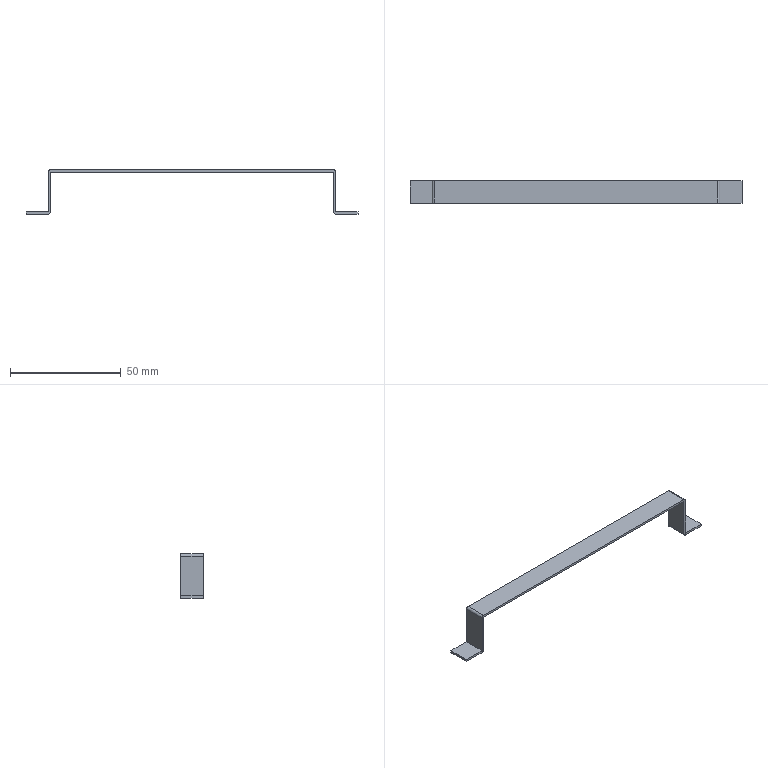Part | STEP file | RJWD-DY-0101_30002 | 1 solid | 18 faces | box 150 x 10 x 20 mm | volume 1872 mm3 | plane 14 | cylinder 4 | commonest cylinder face diameters 2.004 x3 2 x1
STEP:
#1=CARTESIAN_POINT('',(0.,0.,0.));
#2=DIRECTION('',(0.,0.,1.));
#3=DIRECTION('',(1.,0.,0.));
#4=AXIS2_PLACEMENT_3D('',#1,#2,#3);
#5=CARTESIAN_POINT('',(-900.573,5381.573,97.644));
#6=VERTEX_POINT('',#5);
#7=CARTESIAN_POINT('',(-901.573,5381.573,98.644));
#8=VERTEX_POINT('',#7);
#9=CARTESIAN_POINT('',(-901.573,5381.573,97.644));
#10=DIRECTION('',(0.,-1.,0.));
#11=DIRECTION('',(1.,0.,0.));
#12=AXIS2_PLACEMENT_3D('',#9,#10,#11);
#13=CIRCLE('',#12,1.);
#14=CARTESIAN_POINT('',(-1040.573,5381.573,97.644));
#15=DIRECTION('',(0.,-1.,0.));
#16=DIRECTION('',(0.,0.,-1.));
#17=AXIS2_PLACEMENT_3D('',#14,#15,#16);
#18=PLANE('',#17);
#19=CARTESIAN_POINT('',(0.,139.));
#20=DIRECTION('',(0.,1.));
#21=AXIS2_PLACEMENT_2D('',#19,#20);
#22=CIRCLE('',#21,1.);
#23=(GEOMETRIC_REPRESENTATION_CONTEXT(2)PARAMETRIC_REPRESENTATION_CONTEXT()REPRESENTATION_CONTEXT('',''));
#24=DEFINITIONAL_REPRESENTATION('',(#22),#23);
#25=PCURVE('',#18,#24);
#26=CARTESIAN_POINT('',(-901.573,5345.501,97.644));
#27=DIRECTION('',(0.,1.,0.));
#28=DIRECTION('',(0.,0.,1.));
#29=AXIS2_PLACEMENT_3D('',#26,#27,#28);
#30=CYLINDRICAL_SURFACE('',#29,1.);
#31=CARTESIAN_POINT('',(1.571,36.072));
#32=DIRECTION('',(-1.,0.));
#33=VECTOR('',#32,1.);
#34=LINE('',#31,#33);
#35=(GEOMETRIC_REPRESENTATION_CONTEXT(2)PARAMETRIC_REPRESENTATION_CONTEXT()REPRESENTATION_CONTEXT('',''));
#36=DEFINITIONAL_REPRESENTATION('',(#34),#35);
#37=PCURVE('',#30,#36);
#38=SURFACE_CURVE('',#13,(#25,#37),.PCURVE_S1.);
#39=EDGE_CURVE('',#6,#8,#38,.T.);
#40=ORIENTED_EDGE('',*,*,#39,.F.);
#41=CARTESIAN_POINT('',(-900.573,5381.573,79.644));
#42=VERTEX_POINT('',#41);
#43=CARTESIAN_POINT('',(-900.573,5381.573,97.644));
#44=DIRECTION('',(0.,0.,-1.));
#45=VECTOR('',#44,1.);
#46=LINE('',#43,#45);
#47=CARTESIAN_POINT('',(0.,140.));
#48=DIRECTION('',(1.,0.));
#49=VECTOR('',#48,1.);
#50=LINE('',#47,#49);
#51=(GEOMETRIC_REPRESENTATION_CONTEXT(2)PARAMETRIC_REPRESENTATION_CONTEXT()REPRESENTATION_CONTEXT('',''));
#52=DEFINITIONAL_REPRESENTATION('',(#50),#51);
#53=PCURVE('',#18,#52);
#54=CARTESIAN_POINT('',(-900.573,-10.,0.));
#55=DIRECTION('',(1.,0.,0.));
#56=DIRECTION('',(0.,0.,-1.));
#57=AXIS2_PLACEMENT_3D('',#54,#55,#56);
#58=PLANE('',#57);
#59=CARTESIAN_POINT('',(-97.644,5391.573));
#60=DIRECTION('',(1.,0.));
#61=VECTOR('',#60,1.);
#62=LINE('',#59,#61);
#63=(GEOMETRIC_REPRESENTATION_CONTEXT(2)PARAMETRIC_REPRESENTATION_CONTEXT()REPRESENTATION_CONTEXT('',''));
#64=DEFINITIONAL_REPRESENTATION('',(#62),#63);
#65=PCURVE('',#58,#64);
#66=SURFACE_CURVE('',#46,(#53,#65),.PCURVE_S1.);
#67=EDGE_CURVE('',#6,#42,#66,.T.);
#68=ORIENTED_EDGE('',*,*,#67,.T.);
#69=CARTESIAN_POINT('',(-890.573,5381.573,79.644));
#70=VERTEX_POINT('',#69);
#71=CARTESIAN_POINT('',(-890.573,5381.573,79.644));
#72=DIRECTION('',(-1.,0.,0.));
#73=VECTOR('',#72,1.);
#74=LINE('',#71,#73);
#75=CARTESIAN_POINT('',(18.,150.));
#76=DIRECTION('',(0.,-1.));
#77=VECTOR('',#76,1.);
#78=LINE('',#75,#77);
#79=(GEOMETRIC_REPRESENTATION_CONTEXT(2)PARAMETRIC_REPRESENTATION_CONTEXT()REPRESENTATION_CONTEXT('',''));
#80=DEFINITIONAL_REPRESENTATION('',(#78),#79);
#81=PCURVE('',#18,#80);
#82=CARTESIAN_POINT('',(-80.,-10.,79.644));
#83=DIRECTION('',(0.,0.,1.));
#84=DIRECTION('',(1.,0.,0.));
#85=AXIS2_PLACEMENT_3D('',#82,#83,#84);
#86=PLANE('',#85);
#87=CARTESIAN_POINT('',(-810.573,5391.573));
#88=DIRECTION('',(-1.,0.));
#89=VECTOR('',#88,1.);
#90=LINE('',#87,#89);
#91=(GEOMETRIC_REPRESENTATION_CONTEXT(2)PARAMETRIC_REPRESENTATION_CONTEXT()REPRESENTATION_CONTEXT('',''));
#92=DEFINITIONAL_REPRESENTATION('',(#90),#91);
#93=PCURVE('',#86,#92);
#94=SURFACE_CURVE('',#74,(#81,#93),.PCURVE_S1.);
#95=EDGE_CURVE('',#70,#42,#94,.T.);
#96=ORIENTED_EDGE('',*,*,#95,.F.);
#97=CARTESIAN_POINT('',(-890.573,5381.573,78.644));
#98=VERTEX_POINT('',#97);
#99=CARTESIAN_POINT('',(-890.573,5381.573,79.644));
#100=DIRECTION('',(0.,0.,-1.));
#101=VECTOR('',#100,1.);
#102=LINE('',#99,#101);
#103=CARTESIAN_POINT('',(18.,150.));
#104=DIRECTION('',(1.,0.));
#105=VECTOR('',#104,1.);
#106=LINE('',#103,#105);
#107=(GEOMETRIC_REPRESENTATION_CONTEXT(2)PARAMETRIC_REPRESENTATION_CONTEXT()REPRESENTATION_CONTEXT('',''));
#108=DEFINITIONAL_REPRESENTATION('',(#106),#107);
#109=PCURVE('',#18,#108);
#110=CARTESIAN_POINT('',(-890.573,5371.573,78.644));
#111=DIRECTION('',(1.,0.,0.));
#112=DIRECTION('',(0.,0.,-1.));
#113=AXIS2_PLACEMENT_3D('',#110,#111,#112);
#114=PLANE('',#113);
#115=CARTESIAN_POINT('',(-1.,10.));
#116=DIRECTION('',(1.,0.));
#117=VECTOR('',#116,1.);
#118=LINE('',#115,#117);
#119=(GEOMETRIC_REPRESENTATION_CONTEXT(2)PARAMETRIC_REPRESENTATION_CONTEXT()REPRESENTATION_CONTEXT('',''));
#120=DEFINITIONAL_REPRESENTATION('',(#118),#119);
#121=PCURVE('',#114,#120);
#122=SURFACE_CURVE('',#102,(#109,#121),.PCURVE_S1.);
#123=EDGE_CURVE('',#70,#98,#122,.T.);
#124=ORIENTED_EDGE('',*,*,#123,.T.);
#125=CARTESIAN_POINT('',(-900.571,5381.573,78.644));
#126=VERTEX_POINT('',#125);
#127=CARTESIAN_POINT('',(-890.573,5381.573,78.644));
#128=DIRECTION('',(-1.,0.,0.));
#129=VECTOR('',#128,1.);
#130=LINE('',#127,#129);
#131=CARTESIAN_POINT('',(19.,150.));
#132=DIRECTION('',(0.,-1.));
#133=VECTOR('',#132,1.);
#134=LINE('',#131,#133);
#135=(GEOMETRIC_REPRESENTATION_CONTEXT(2)PARAMETRIC_REPRESENTATION_CONTEXT()REPRESENTATION_CONTEXT('',''));
#136=DEFINITIONAL_REPRESENTATION('',(#134),#135);
#137=PCURVE('',#18,#136);
#138=CARTESIAN_POINT('',(-80.,-10.,78.644));
#139=DIRECTION('',(0.,0.,1.));
#140=DIRECTION('',(1.,0.,0.));
#141=AXIS2_PLACEMENT_3D('',#138,#139,#140);
#142=PLANE('',#141);
#143=CARTESIAN_POINT('',(-810.573,5391.573));
#144=DIRECTION('',(-1.,0.));
#145=VECTOR('',#144,1.);
#146=LINE('',#143,#145);
#147=(GEOMETRIC_REPRESENTATION_CONTEXT(2)PARAMETRIC_REPRESENTATION_CONTEXT()REPRESENTATION_CONTEXT('',''));
#148=DEFINITIONAL_REPRESENTATION('',(#146),#147);
#149=PCURVE('',#142,#148);
#150=SURFACE_CURVE('',#130,(#137,#149),.PCURVE_S1.);
#151=EDGE_CURVE('',#98,#126,#150,.T.);
#152=ORIENTED_EDGE('',*,*,#151,.T.);
#153=CARTESIAN_POINT('',(-901.573,5381.573,79.646));
#154=VERTEX_POINT('',#153);
#155=CARTESIAN_POINT('',(-900.571,5381.573,79.646));
#156=DIRECTION('',(0.,-1.,0.));
#157=DIRECTION('',(-1.,0.,0.));
#158=AXIS2_PLACEMENT_3D('',#155,#156,#157);
#159=CIRCLE('',#158,1.002);
#160=CARTESIAN_POINT('',(17.998,140.002));
#161=DIRECTION('',(0.,-1.));
#162=AXIS2_PLACEMENT_2D('',#160,#161);
#163=CIRCLE('',#162,1.002);
#164=(GEOMETRIC_REPRESENTATION_CONTEXT(2)PARAMETRIC_REPRESENTATION_CONTEXT()REPRESENTATION_CONTEXT('',''));
#165=DEFINITIONAL_REPRESENTATION('',(#163),#164);
#166=PCURVE('',#18,#165);
#167=CARTESIAN_POINT('',(-900.571,5411.573,79.646));
#168=DIRECTION('',(0.,-1.,0.));
#169=DIRECTION('',(1.,0.,0.));
#170=AXIS2_PLACEMENT_3D('',#167,#168,#169);
#171=CYLINDRICAL_SURFACE('',#170,1.002);
#172=CARTESIAN_POINT('',(3.142,30.));
#173=DIRECTION('',(1.,0.));
#174=VECTOR('',#173,1.);
#175=LINE('',#172,#174);
#176=(GEOMETRIC_REPRESENTATION_CONTEXT(2)PARAMETRIC_REPRESENTATION_CONTEXT()REPRESENTATION_CONTEXT('',''));
#177=DEFINITIONAL_REPRESENTATION('',(#175),#176);
#178=PCURVE('',#171,#177);
#179=SURFACE_CURVE('',#159,(#166,#178),.PCURVE_S1.);
#180=EDGE_CURVE('',#154,#126,#179,.T.);
#181=ORIENTED_EDGE('',*,*,#180,.F.);
#182=CARTESIAN_POINT('',(-901.573,5381.573,97.644));
#183=VERTEX_POINT('',#182);
#184=CARTESIAN_POINT('',(-901.573,5381.573,79.646));
#185=DIRECTION('',(0.,0.,1.));
#186=VECTOR('',#185,1.);
#187=LINE('',#184,#186);
#188=CARTESIAN_POINT('',(17.998,139.));
#189=DIRECTION('',(-1.,0.));
#190=VECTOR('',#189,1.);
#191=LINE('',#188,#190);
#192=(GEOMETRIC_REPRESENTATION_CONTEXT(2)PARAMETRIC_REPRESENTATION_CONTEXT()REPRESENTATION_CONTEXT('',''));
#193=DEFINITIONAL_REPRESENTATION('',(#191),#192);
#194=PCURVE('',#18,#193);
#195=CARTESIAN_POINT('',(-901.573,-10.,0.));
#196=DIRECTION('',(1.,0.,0.));
#197=DIRECTION('',(0.,0.,-1.));
#198=AXIS2_PLACEMENT_3D('',#195,#196,#197);
#199=PLANE('',#198);
#200=CARTESIAN_POINT('',(-79.646,5391.573));
#201=DIRECTION('',(-1.,0.));
#202=VECTOR('',#201,1.);
#203=LINE('',#200,#202);
#204=(GEOMETRIC_REPRESENTATION_CONTEXT(2)PARAMETRIC_REPRESENTATION_CONTEXT()REPRESENTATION_CONTEXT('',''));
#205=DEFINITIONAL_REPRESENTATION('',(#203),#204);
#206=PCURVE('',#199,#205);
#207=SURFACE_CURVE('',#187,(#194,#206),.PCURVE_S1.);
#208=EDGE_CURVE('',#154,#183,#207,.T.);
#209=ORIENTED_EDGE('',*,*,#208,.T.);
#210=CARTESIAN_POINT('',(-1029.573,5381.573,97.644));
#211=VERTEX_POINT('',#210);
#212=CARTESIAN_POINT('',(-901.573,5381.573,97.644));
#213=DIRECTION('',(-1.,0.,0.));
#214=VECTOR('',#213,1.);
#215=LINE('',#212,#214);
#216=CARTESIAN_POINT('',(0.,139.));
#217=DIRECTION('',(0.,-1.));
#218=VECTOR('',#217,1.);
#219=LINE('',#216,#218);
#220=(GEOMETRIC_REPRESENTATION_CONTEXT(2)PARAMETRIC_REPRESENTATION_CONTEXT()REPRESENTATION_CONTEXT('',''));
#221=DEFINITIONAL_REPRESENTATION('',(#219),#220);
#222=PCURVE('',#18,#221);
#223=CARTESIAN_POINT('',(0.,-10.,97.644));
#224=DIRECTION('',(0.,0.,1.));
#225=DIRECTION('',(1.,0.,0.));
#226=AXIS2_PLACEMENT_3D('',#223,#224,#225);
#227=PLANE('',#226);
#228=CARTESIAN_POINT('',(-901.573,5391.573));
#229=DIRECTION('',(-1.,0.));
#230=VECTOR('',#229,1.);
#231=LINE('',#228,#230);
#232=(GEOMETRIC_REPRESENTATION_CONTEXT(2)PARAMETRIC_REPRESENTATION_CONTEXT()REPRESENTATION_CONTEXT('',''));
#233=DEFINITIONAL_REPRESENTATION('',(#231),#232);
#234=PCURVE('',#227,#233);
#235=SURFACE_CURVE('',#215,(#222,#234),.PCURVE_S1.);
#236=EDGE_CURVE('',#183,#211,#235,.T.);
#237=ORIENTED_EDGE('',*,*,#236,.T.);
#238=CARTESIAN_POINT('',(-1029.573,5381.573,79.646));
#239=VERTEX_POINT('',#238);
#240=CARTESIAN_POINT('',(-1029.573,5381.573,79.646));
#241=DIRECTION('',(0.,0.,1.));
#242=VECTOR('',#241,1.);
#243=LINE('',#240,#242);
#244=CARTESIAN_POINT('',(17.998,11.));
#245=DIRECTION('',(-1.,0.));
#246=VECTOR('',#245,1.);
#247=LINE('',#244,#246);
#248=(GEOMETRIC_REPRESENTATION_CONTEXT(2)PARAMETRIC_REPRESENTATION_CONTEXT()REPRESENTATION_CONTEXT('',''));
#249=DEFINITIONAL_REPRESENTATION('',(#247),#248);
#250=PCURVE('',#18,#249);
#251=CARTESIAN_POINT('',(-1029.573,-10.,0.));
#252=DIRECTION('',(1.,0.,0.));
#253=DIRECTION('',(0.,0.,-1.));
#254=AXIS2_PLACEMENT_3D('',#251,#252,#253);
#255=PLANE('',#254);
#256=CARTESIAN_POINT('',(-79.646,5391.573));
#257=DIRECTION('',(-1.,0.));
#258=VECTOR('',#257,1.);
#259=LINE('',#256,#258);
#260=(GEOMETRIC_REPRESENTATION_CONTEXT(2)PARAMETRIC_REPRESENTATION_CONTEXT()REPRESENTATION_CONTEXT('',''));
#261=DEFINITIONAL_REPRESENTATION('',(#259),#260);
#262=PCURVE('',#255,#261);
#263=SURFACE_CURVE('',#243,(#250,#262),.PCURVE_S1.);
#264=EDGE_CURVE('',#239,#211,#263,.T.);
#265=ORIENTED_EDGE('',*,*,#264,.F.);
#266=CARTESIAN_POINT('',(-1030.575,5381.573,78.644));
#267=VERTEX_POINT('',#266);
#268=CARTESIAN_POINT('',(-1030.575,5381.573,79.646));
#269=DIRECTION('',(0.,-1.,0.));
#270=DIRECTION('',(0.,0.,-1.));
#271=AXIS2_PLACEMENT_3D('',#268,#269,#270);
#272=CIRCLE('',#271,1.002);
#273=CARTESIAN_POINT('',(17.998,9.998));
#274=DIRECTION('',(1.,0.));
#275=AXIS2_PLACEMENT_2D('',#273,#274);
#276=CIRCLE('',#275,1.002);
#277=(GEOMETRIC_REPRESENTATION_CONTEXT(2)PARAMETRIC_REPRESENTATION_CONTEXT()REPRESENTATION_CONTEXT('',''));
#278=DEFINITIONAL_REPRESENTATION('',(#276),#277);
#279=PCURVE('',#18,#278);
#280=CARTESIAN_POINT('',(-1030.575,5371.573,79.646));
#281=DIRECTION('',(0.,1.,0.));
#282=DIRECTION('',(-1.,0.,0.));
#283=AXIS2_PLACEMENT_3D('',#280,#281,#282);
#284=CYLINDRICAL_SURFACE('',#283,1.002);
#285=CARTESIAN_POINT('',(4.712,10.));
#286=DIRECTION('',(-1.,0.));
#287=VECTOR('',#286,1.);
#288=LINE('',#285,#287);
#289=(GEOMETRIC_REPRESENTATION_CONTEXT(2)PARAMETRIC_REPRESENTATION_CONTEXT()REPRESENTATION_CONTEXT('',''));
#290=DEFINITIONAL_REPRESENTATION('',(#288),#289);
#291=PCURVE('',#284,#290);
#292=SURFACE_CURVE('',#272,(#279,#291),.PCURVE_S1.);
#293=EDGE_CURVE('',#267,#239,#292,.T.);
#294=ORIENTED_EDGE('',*,*,#293,.F.);
#295=CARTESIAN_POINT('',(-1040.573,5381.573,78.644));
#296=VERTEX_POINT('',#295);
#297=CARTESIAN_POINT('',(-1040.573,5381.573,78.644));
#298=DIRECTION('',(1.,0.,0.));
#299=VECTOR('',#298,1.);
#300=LINE('',#297,#299);
#301=CARTESIAN_POINT('',(19.,0.));
#302=DIRECTION('',(0.,1.));
#303=VECTOR('',#302,1.);
#304=LINE('',#301,#303);
#305=(GEOMETRIC_REPRESENTATION_CONTEXT(2)PARAMETRIC_REPRESENTATION_CONTEXT()REPRESENTATION_CONTEXT('',''));
#306=DEFINITIONAL_REPRESENTATION('',(#304),#305);
#307=PCURVE('',#18,#306);
#308=CARTESIAN_POINT('',(10.,-10.,78.644));
#309=DIRECTION('',(0.,0.,-1.));
#310=DIRECTION('',(-1.,0.,0.));
#311=AXIS2_PLACEMENT_3D('',#308,#309,#310);
#312=PLANE('',#311);
#313=CARTESIAN_POINT('',(1050.573,5391.573));
#314=DIRECTION('',(-1.,0.));
#315=VECTOR('',#314,1.);
#316=LINE('',#313,#315);
#317=(GEOMETRIC_REPRESENTATION_CONTEXT(2)PARAMETRIC_REPRESENTATION_CONTEXT()REPRESENTATION_CONTEXT('',''));
#318=DEFINITIONAL_REPRESENTATION('',(#316),#317);
#319=PCURVE('',#312,#318);
#320=SURFACE_CURVE('',#300,(#307,#319),.PCURVE_S1.);
#321=EDGE_CURVE('',#296,#267,#320,.T.);
#322=ORIENTED_EDGE('',*,*,#321,.F.);
#323=CARTESIAN_POINT('',(-1040.573,5381.573,79.644));
#324=VERTEX_POINT('',#323);
#325=CARTESIAN_POINT('',(-1040.573,5381.573,79.644));
#326=DIRECTION('',(0.,0.,-1.));
#327=VECTOR('',#326,1.);
#328=LINE('',#325,#327);
#329=CARTESIAN_POINT('',(18.,0.));
#330=DIRECTION('',(1.,0.));
#331=VECTOR('',#330,1.);
#332=LINE('',#329,#331);
#333=(GEOMETRIC_REPRESENTATION_CONTEXT(2)PARAMETRIC_REPRESENTATION_CONTEXT()REPRESENTATION_CONTEXT('',''));
#334=DEFINITIONAL_REPRESENTATION('',(#332),#333);
#335=PCURVE('',#18,#334);
#336=CARTESIAN_POINT('',(-1040.573,5371.573,78.644));
#337=DIRECTION('',(1.,0.,0.));
#338=DIRECTION('',(0.,0.,-1.));
#339=AXIS2_PLACEMENT_3D('',#336,#337,#338);
#340=PLANE('',#339);
#341=CARTESIAN_POINT('',(-1.,10.));
#342=DIRECTION('',(1.,0.));
#343=VECTOR('',#342,1.);
#344=LINE('',#341,#343);
#345=(GEOMETRIC_REPRESENTATION_CONTEXT(2)PARAMETRIC_REPRESENTATION_CONTEXT()REPRESENTATION_CONTEXT('',''));
#346=DEFINITIONAL_REPRESENTATION('',(#344),#345);
#347=PCURVE('',#340,#346);
#348=SURFACE_CURVE('',#328,(#335,#347),.PCURVE_S1.);
#349=EDGE_CURVE('',#324,#296,#348,.T.);
#350=ORIENTED_EDGE('',*,*,#349,.F.);
#351=CARTESIAN_POINT('',(-1030.573,5381.573,79.644));
#352=VERTEX_POINT('',#351);
#353=CARTESIAN_POINT('',(-1040.573,5381.573,79.644));
#354=DIRECTION('',(1.,0.,0.));
#355=VECTOR('',#354,1.);
#356=LINE('',#353,#355);
#357=CARTESIAN_POINT('',(18.,0.));
#358=DIRECTION('',(0.,1.));
#359=VECTOR('',#358,1.);
#360=LINE('',#357,#359);
#361=(GEOMETRIC_REPRESENTATION_CONTEXT(2)PARAMETRIC_REPRESENTATION_CONTEXT()REPRESENTATION_CONTEXT('',''));
#362=DEFINITIONAL_REPRESENTATION('',(#360),#361);
#363=PCURVE('',#18,#362);
#364=CARTESIAN_POINT('',(10.,-10.,79.644));
#365=DIRECTION('',(0.,0.,-1.));
#366=DIRECTION('',(-1.,0.,0.));
#367=AXIS2_PLACEMENT_3D('',#364,#365,#366);
#368=PLANE('',#367);
#369=CARTESIAN_POINT('',(1050.573,5391.573));
#370=DIRECTION('',(-1.,0.));
#371=VECTOR('',#370,1.);
#372=LINE('',#369,#371);
#373=(GEOMETRIC_REPRESENTATION_CONTEXT(2)PARAMETRIC_REPRESENTATION_CONTEXT()REPRESENTATION_CONTEXT('',''));
#374=DEFINITIONAL_REPRESENTATION('',(#372),#373);
#375=PCURVE('',#368,#374);
#376=SURFACE_CURVE('',#356,(#363,#375),.PCURVE_S1.);
#377=EDGE_CURVE('',#324,#352,#376,.T.);
#378=ORIENTED_EDGE('',*,*,#377,.T.);
#379=CARTESIAN_POINT('',(-1030.573,5381.573,97.642));
#380=VERTEX_POINT('',#379);
#381=CARTESIAN_POINT('',(-1030.573,5381.573,79.644));
#382=DIRECTION('',(0.,0.,1.));
#383=VECTOR('',#382,1.);
#384=LINE('',#381,#383);
#385=CARTESIAN_POINT('',(18.,10.));
#386=DIRECTION('',(-1.,0.));
#387=VECTOR('',#386,1.);
#388=LINE('',#385,#387);
#389=(GEOMETRIC_REPRESENTATION_CONTEXT(2)PARAMETRIC_REPRESENTATION_CONTEXT()REPRESENTATION_CONTEXT('',''));
#390=DEFINITIONAL_REPRESENTATION('',(#388),#389);
#391=PCURVE('',#18,#390);
#392=CARTESIAN_POINT('',(-1030.573,-10.,0.));
#393=DIRECTION('',(1.,0.,0.));
#394=DIRECTION('',(0.,0.,-1.));
#395=AXIS2_PLACEMENT_3D('',#392,#393,#394);
#396=PLANE('',#395);
#397=CARTESIAN_POINT('',(-79.644,5391.573));
#398=DIRECTION('',(-1.,0.));
#399=VECTOR('',#398,1.);
#400=LINE('',#397,#399);
#401=(GEOMETRIC_REPRESENTATION_CONTEXT(2)PARAMETRIC_REPRESENTATION_CONTEXT()REPRESENTATION_CONTEXT('',''));
#402=DEFINITIONAL_REPRESENTATION('',(#400),#401);
#403=PCURVE('',#396,#402);
#404=SURFACE_CURVE('',#384,(#391,#403),.PCURVE_S1.);
#405=EDGE_CURVE('',#352,#380,#404,.T.);
#406=ORIENTED_EDGE('',*,*,#405,.T.);
#407=CARTESIAN_POINT('',(-1029.571,5381.573,98.644));
#408=VERTEX_POINT('',#407);
#409=CARTESIAN_POINT('',(-1029.571,5381.573,97.642));
#410=DIRECTION('',(0.,-1.,0.));
#411=DIRECTION('',(0.,0.,1.));
#412=AXIS2_PLACEMENT_3D('',#409,#410,#411);
#413=CIRCLE('',#412,1.002);
#414=CARTESIAN_POINT('',(0.002,11.002));
#415=DIRECTION('',(-1.,0.));
#416=AXIS2_PLACEMENT_2D('',#414,#415);
#417=CIRCLE('',#416,1.002);
#418=(GEOMETRIC_REPRESENTATION_CONTEXT(2)PARAMETRIC_REPRESENTATION_CONTEXT()REPRESENTATION_CONTEXT('',''));
#419=DEFINITIONAL_REPRESENTATION('',(#417),#418);
#420=PCURVE('',#18,#419);
#421=CARTESIAN_POINT('',(-1029.571,5411.573,97.642));
#422=DIRECTION('',(0.,-1.,0.));
#423=DIRECTION('',(0.,0.,-1.));
#424=AXIS2_PLACEMENT_3D('',#421,#422,#423);
#425=CYLINDRICAL_SURFACE('',#424,1.002);
#426=CARTESIAN_POINT('',(3.142,30.));
#427=DIRECTION('',(1.,0.));
#428=VECTOR('',#427,1.);
#429=LINE('',#426,#428);
#430=(GEOMETRIC_REPRESENTATION_CONTEXT(2)PARAMETRIC_REPRESENTATION_CONTEXT()REPRESENTATION_CONTEXT('',''));
#431=DEFINITIONAL_REPRESENTATION('',(#429),#430);
#432=PCURVE('',#425,#431);
#433=SURFACE_CURVE('',#413,(#420,#432),.PCURVE_S1.);
#434=EDGE_CURVE('',#408,#380,#433,.T.);
#435=ORIENTED_EDGE('',*,*,#434,.F.);
#436=CARTESIAN_POINT('',(-1029.571,5381.573,98.644));
#437=DIRECTION('',(1.,0.,0.));
#438=VECTOR('',#437,1.);
#439=LINE('',#436,#438);
#440=CARTESIAN_POINT('',(-1.,11.002));
#441=DIRECTION('',(0.,1.));
#442=VECTOR('',#441,1.);
#443=LINE('',#440,#442);
#444=(GEOMETRIC_REPRESENTATION_CONTEXT(2)PARAMETRIC_REPRESENTATION_CONTEXT()REPRESENTATION_CONTEXT('',''));
#445=DEFINITIONAL_REPRESENTATION('',(#443),#444);
#446=PCURVE('',#18,#445);
#447=CARTESIAN_POINT('',(0.,-10.,98.644));
#448=DIRECTION('',(0.,0.,1.));
#449=DIRECTION('',(1.,0.,0.));
#450=AXIS2_PLACEMENT_3D('',#447,#448,#449);
#451=PLANE('',#450);
#452=CARTESIAN_POINT('',(-1029.571,5391.573));
#453=DIRECTION('',(1.,0.));
#454=VECTOR('',#453,1.);
#455=LINE('',#452,#454);
#456=(GEOMETRIC_REPRESENTATION_CONTEXT(2)PARAMETRIC_REPRESENTATION_CONTEXT()REPRESENTATION_CONTEXT('',''));
#457=DEFINITIONAL_REPRESENTATION('',(#455),#456);
#458=PCURVE('',#451,#457);
#459=SURFACE_CURVE('',#439,(#446,#458),.PCURVE_S1.);
#460=EDGE_CURVE('',#408,#8,#459,.T.);
#461=ORIENTED_EDGE('',*,*,#460,.T.);
#462=EDGE_LOOP('',(#40,#68,#96,#124,#152,#181,#209,#237,#265,#294,#322,#350,#378,#406,#435,#461));
#463=FACE_BOUND('',#462,.F.);
#464=ADVANCED_FACE('',(#463),#18,.T.);
#465=CARTESIAN_POINT('',(-901.573,5391.573,98.644));
#466=VERTEX_POINT('',#465);
#467=CARTESIAN_POINT('',(-901.573,5381.573,98.644));
#468=DIRECTION('',(0.,1.,0.));
#469=VECTOR('',#468,1.);
#470=LINE('',#467,#469);
#471=CARTESIAN_POINT('',(0.,36.072));
#472=DIRECTION('',(0.,1.));
#473=VECTOR('',#472,1.);
#474=LINE('',#471,#473);
#475=(GEOMETRIC_REPRESENTATION_CONTEXT(2)PARAMETRIC_REPRESENTATION_CONTEXT()REPRESENTATION_CONTEXT('',''));
#476=DEFINITIONAL_REPRESENTATION('',(#474),#475);
#477=PCURVE('',#30,#476);
#478=CARTESIAN_POINT('',(-901.573,5391.573));
#479=DIRECTION('',(0.,1.));
#480=VECTOR('',#479,1.);
#481=LINE('',#478,#480);
#482=(GEOMETRIC_REPRESENTATION_CONTEXT(2)PARAMETRIC_REPRESENTATION_CONTEXT()REPRESENTATION_CONTEXT('',''));
#483=DEFINITIONAL_REPRESENTATION('',(#481),#482);
#484=PCURVE('',#451,#483);
#485=SURFACE_CURVE('',#470,(#477,#484),.PCURVE_S1.);
#486=EDGE_CURVE('',#8,#466,#485,.T.);
#487=ORIENTED_EDGE('',*,*,#486,.F.);
#488=ORIENTED_EDGE('',*,*,#39,.F.);
#489=CARTESIAN_POINT('',(-900.573,5391.573,97.644));
#490=VERTEX_POINT('',#489);
#491=CARTESIAN_POINT('',(-900.573,5381.573,97.644));
#492=DIRECTION('',(0.,1.,0.));
#493=VECTOR('',#492,1.);
#494=LINE('',#491,#493);
#495=CARTESIAN_POINT('',(1.571,36.072));
#496=DIRECTION('',(0.,1.));
#497=VECTOR('',#496,1.);
#498=LINE('',#495,#497);
#499=(GEOMETRIC_REPRESENTATION_CONTEXT(2)PARAMETRIC_REPRESENTATION_CONTEXT()REPRESENTATION_CONTEXT('',''));
#500=DEFINITIONAL_REPRESENTATION('',(#498),#499);
#501=PCURVE('',#30,#500);
#502=CARTESIAN_POINT('',(-97.644,5391.573));
#503=DIRECTION('',(0.,1.));
#504=VECTOR('',#503,1.);
#505=LINE('',#502,#504);
#506=(GEOMETRIC_REPRESENTATION_CONTEXT(2)PARAMETRIC_REPRESENTATION_CONTEXT()REPRESENTATION_CONTEXT('',''));
#507=DEFINITIONAL_REPRESENTATION('',(#505),#506);
#508=PCURVE('',#58,#507);
#509=SURFACE_CURVE('',#494,(#501,#508),.PCURVE_S1.);
#510=EDGE_CURVE('',#6,#490,#509,.T.);
#511=ORIENTED_EDGE('',*,*,#510,.T.);
#512=CARTESIAN_POINT('',(-901.573,5391.573,97.644));
#513=DIRECTION('',(0.,1.,0.));
#514=DIRECTION('',(0.,0.,1.));
#515=AXIS2_PLACEMENT_3D('',#512,#513,#514);
#516=CIRCLE('',#515,1.);
#517=CARTESIAN_POINT('',(0.,46.072));
#518=DIRECTION('',(1.,0.));
#519=VECTOR('',#518,1.);
#520=LINE('',#517,#519);
#521=(GEOMETRIC_REPRESENTATION_CONTEXT(2)PARAMETRIC_REPRESENTATION_CONTEXT()REPRESENTATION_CONTEXT('',''));
#522=DEFINITIONAL_REPRESENTATION('',(#520),#521);
#523=PCURVE('',#30,#522);
#524=CARTESIAN_POINT('',(-820.573,5391.573,97.644));
#525=DIRECTION('',(0.,1.,0.));
#526=DIRECTION('',(0.,0.,1.));
#527=AXIS2_PLACEMENT_3D('',#524,#525,#526);
#528=PLANE('',#527);
#529=CARTESIAN_POINT('',(0.,-81.));
#530=DIRECTION('',(1.,0.));
#531=AXIS2_PLACEMENT_2D('',#529,#530);
#532=CIRCLE('',#531,1.);
#533=(GEOMETRIC_REPRESENTATION_CONTEXT(2)PARAMETRIC_REPRESENTATION_CONTEXT()REPRESENTATION_CONTEXT('',''));
#534=DEFINITIONAL_REPRESENTATION('',(#532),#533);
#535=PCURVE('',#528,#534);
#536=SURFACE_CURVE('',#516,(#523,#535),.PCURVE_S1.);
#537=EDGE_CURVE('',#466,#490,#536,.T.);
#538=ORIENTED_EDGE('',*,*,#537,.F.);
#539=EDGE_LOOP('',(#487,#488,#511,#538));
#540=FACE_BOUND('',#539,.T.);
#541=ADVANCED_FACE('',(#540),#30,.T.);
#542=ORIENTED_EDGE('',*,*,#537,.F.);
#543=CARTESIAN_POINT('',(-1029.571,5391.573,98.644));
#544=VERTEX_POINT('',#543);
#545=CARTESIAN_POINT('',(-901.573,5391.573,98.644));
#546=DIRECTION('',(-1.,0.,0.));
#547=VECTOR('',#546,1.);
#548=LINE('',#545,#547);
#549=CARTESIAN_POINT('',(1.,-81.));
#550=DIRECTION('',(0.,-1.));
#551=VECTOR('',#550,1.);
#552=LINE('',#549,#551);
#553=(GEOMETRIC_REPRESENTATION_CONTEXT(2)PARAMETRIC_REPRESENTATION_CONTEXT()REPRESENTATION_CONTEXT('',''));
#554=DEFINITIONAL_REPRESENTATION('',(#552),#553);
#555=PCURVE('',#528,#554);
#556=CARTESIAN_POINT('',(-901.573,5401.573));
#557=DIRECTION('',(-1.,0.));
#558=VECTOR('',#557,1.);
#559=LINE('',#556,#558);
#560=(GEOMETRIC_REPRESENTATION_CONTEXT(2)PARAMETRIC_REPRESENTATION_CONTEXT()REPRESENTATION_CONTEXT('',''));
#561=DEFINITIONAL_REPRESENTATION('',(#559),#560);
#562=PCURVE('',#451,#561);
#563=SURFACE_CURVE('',#548,(#555,#562),.PCURVE_S1.);
#564=EDGE_CURVE('',#466,#544,#563,.T.);
#565=ORIENTED_EDGE('',*,*,#564,.T.);
#566=CARTESIAN_POINT('',(-1030.573,5391.573,97.642));
#567=VERTEX_POINT('',#566);
#568=CARTESIAN_POINT('',(-1029.571,5391.573,97.642));
#569=DIRECTION('',(0.,1.,0.));
#570=DIRECTION('',(-1.,0.,0.));
#571=AXIS2_PLACEMENT_3D('',#568,#569,#570);
#572=CIRCLE('',#571,1.002);
#573=CARTESIAN_POINT('',(-0.002,-208.998));
#574=DIRECTION('',(0.,-1.));
#575=AXIS2_PLACEMENT_2D('',#573,#574);
#576=CIRCLE('',#575,1.002);
#577=(GEOMETRIC_REPRESENTATION_CONTEXT(2)PARAMETRIC_REPRESENTATION_CONTEXT()REPRESENTATION_CONTEXT('',''));
#578=DEFINITIONAL_REPRESENTATION('',(#576),#577);
#579=PCURVE('',#528,#578);
#580=CARTESIAN_POINT('',(4.712,20.));
#581=DIRECTION('',(-1.,0.));
#582=VECTOR('',#581,1.);
#583=LINE('',#580,#582);
#584=(GEOMETRIC_REPRESENTATION_CONTEXT(2)PARAMETRIC_REPRESENTATION_CONTEXT()REPRESENTATION_CONTEXT('',''));
#585=DEFINITIONAL_REPRESENTATION('',(#583),#584);
#586=PCURVE('',#425,#585);
#587=SURFACE_CURVE('',#572,(#579,#586),.PCURVE_S1.);
#588=EDGE_CURVE('',#567,#544,#587,.T.);
#589=ORIENTED_EDGE('',*,*,#588,.F.);
#590=CARTESIAN_POINT('',(-1030.573,5391.573,79.644));
#591=VERTEX_POINT('',#590);
#592=CARTESIAN_POINT('',(-1030.573,5391.573,97.642));
#593=DIRECTION('',(-0.00003704,0.,-1.));
#594=VECTOR('',#593,1.);
#595=LINE('',#592,#594);
#596=CARTESIAN_POINT('',(-0.002,-210.));
#597=DIRECTION('',(-1.,-0.00003704));
#598=VECTOR('',#597,1.);
#599=LINE('',#596,#598);
#600=(GEOMETRIC_REPRESENTATION_CONTEXT(2)PARAMETRIC_REPRESENTATION_CONTEXT()REPRESENTATION_CONTEXT('',''));
#601=DEFINITIONAL_REPRESENTATION('',(#599),#600);
#602=PCURVE('',#528,#601);
#603=CARTESIAN_POINT('',(-97.642,5401.573));
#604=DIRECTION('',(1.,0.));
#605=VECTOR('',#604,1.);
#606=LINE('',#603,#605);
#607=(GEOMETRIC_REPRESENTATION_CONTEXT(2)PARAMETRIC_REPRESENTATION_CONTEXT()REPRESENTATION_CONTEXT('',''));
#608=DEFINITIONAL_REPRESENTATION('',(#606),#607);
#609=PCURVE('',#396,#608);
#610=SURFACE_CURVE('',#595,(#602,#609),.PCURVE_S1.);
#611=EDGE_CURVE('',#567,#591,#610,.T.);
#612=ORIENTED_EDGE('',*,*,#611,.T.);
#613=CARTESIAN_POINT('',(-1040.573,5391.573,79.644));
#614=VERTEX_POINT('',#613);
#615=CARTESIAN_POINT('',(-1030.573,5391.573,79.644));
#616=DIRECTION('',(-1.,0.,-0.00006667));
#617=VECTOR('',#616,1.);
#618=LINE('',#615,#617);
#619=CARTESIAN_POINT('',(-17.999,-210.001));
#620=DIRECTION('',(-0.00006667,-1.));
#621=VECTOR('',#620,1.);
#622=LINE('',#619,#621);
#623=(GEOMETRIC_REPRESENTATION_CONTEXT(2)PARAMETRIC_REPRESENTATION_CONTEXT()REPRESENTATION_CONTEXT('',''));
#624=DEFINITIONAL_REPRESENTATION('',(#622),#623);
#625=PCURVE('',#528,#624);
#626=CARTESIAN_POINT('',(1040.573,5401.573));
#627=DIRECTION('',(1.,0.));
#628=VECTOR('',#627,1.);
#629=LINE('',#626,#628);
#630=(GEOMETRIC_REPRESENTATION_CONTEXT(2)PARAMETRIC_REPRESENTATION_CONTEXT()REPRESENTATION_CONTEXT('',''));
#631=DEFINITIONAL_REPRESENTATION('',(#629),#630);
#632=PCURVE('',#368,#631);
#633=SURFACE_CURVE('',#618,(#625,#632),.PCURVE_S1.);
#634=EDGE_CURVE('',#591,#614,#633,.T.);
#635=ORIENTED_EDGE('',*,*,#634,.T.);
#636=CARTESIAN_POINT('',(-1040.573,5391.573,78.644));
#637=VERTEX_POINT('',#636);
#638=CARTESIAN_POINT('',(-1040.573,5391.573,79.644));
#639=DIRECTION('',(0.,0.,-1.));
#640=VECTOR('',#639,1.);
#641=LINE('',#638,#640);
#642=CARTESIAN_POINT('',(-18.,-220.));
#643=DIRECTION('',(-1.,0.));
#644=VECTOR('',#643,1.);
#645=LINE('',#642,#644);
#646=(GEOMETRIC_REPRESENTATION_CONTEXT(2)PARAMETRIC_REPRESENTATION_CONTEXT()REPRESENTATION_CONTEXT('',''));
#647=DEFINITIONAL_REPRESENTATION('',(#645),#646);
#648=PCURVE('',#528,#647);
#649=CARTESIAN_POINT('',(-1.,20.));
#650=DIRECTION('',(1.,0.));
#651=VECTOR('',#650,1.);
#652=LINE('',#649,#651);
#653=(GEOMETRIC_REPRESENTATION_CONTEXT(2)PARAMETRIC_REPRESENTATION_CONTEXT()REPRESENTATION_CONTEXT('',''));
#654=DEFINITIONAL_REPRESENTATION('',(#652),#653);
#655=PCURVE('',#340,#654);
#656=SURFACE_CURVE('',#641,(#648,#655),.PCURVE_S1.);
#657=EDGE_CURVE('',#614,#637,#656,.T.);
#658=ORIENTED_EDGE('',*,*,#657,.T.);
#659=CARTESIAN_POINT('',(-1030.575,5391.573,78.644));
#660=VERTEX_POINT('',#659);
#661=CARTESIAN_POINT('',(-1030.575,5391.573,78.644));
#662=DIRECTION('',(-1.,0.,0.));
#663=VECTOR('',#662,1.);
#664=LINE('',#661,#663);
#665=CARTESIAN_POINT('',(-19.,-210.002));
#666=DIRECTION('',(0.,-1.));
#667=VECTOR('',#666,1.);
#668=LINE('',#665,#667);
#669=(GEOMETRIC_REPRESENTATION_CONTEXT(2)PARAMETRIC_REPRESENTATION_CONTEXT()REPRESENTATION_CONTEXT('',''));
#670=DEFINITIONAL_REPRESENTATION('',(#668),#669);
#671=PCURVE('',#528,#670);
#672=CARTESIAN_POINT('',(1040.575,5401.573));
#673=DIRECTION('',(1.,0.));
#674=VECTOR('',#673,1.);
#675=LINE('',#672,#674);
#676=(GEOMETRIC_REPRESENTATION_CONTEXT(2)PARAMETRIC_REPRESENTATION_CONTEXT()REPRESENTATION_CONTEXT('',''));
#677=DEFINITIONAL_REPRESENTATION('',(#675),#676);
#678=PCURVE('',#312,#677);
#679=SURFACE_CURVE('',#664,(#671,#678),.PCURVE_S1.);
#680=EDGE_CURVE('',#660,#637,#679,.T.);
#681=ORIENTED_EDGE('',*,*,#680,.F.);
#682=CARTESIAN_POINT('',(-1029.573,5391.573,79.646));
#683=VERTEX_POINT('',#682);
#684=CARTESIAN_POINT('',(-1030.575,5391.573,79.646));
#685=DIRECTION('',(0.,1.,0.));
#686=DIRECTION('',(1.,0.,0.));
#687=AXIS2_PLACEMENT_3D('',#684,#685,#686);
#688=CIRCLE('',#687,1.002);
#689=CARTESIAN_POINT('',(-17.998,-210.002));
#690=DIRECTION('',(0.,1.));
#691=AXIS2_PLACEMENT_2D('',#689,#690);
#692=CIRCLE('',#691,1.002);
#693=(GEOMETRIC_REPRESENTATION_CONTEXT(2)PARAMETRIC_REPRESENTATION_CONTEXT()REPRESENTATION_CONTEXT('',''));
#694=DEFINITIONAL_REPRESENTATION('',(#692),#693);
#695=PCURVE('',#528,#694);
#696=CARTESIAN_POINT('',(3.142,20.));
#697=DIRECTION('',(1.,0.));
#698=VECTOR('',#697,1.);
#699=LINE('',#696,#698);
#700=(GEOMETRIC_REPRESENTATION_CONTEXT(2)PARAMETRIC_REPRESENTATION_CONTEXT()REPRESENTATION_CONTEXT('',''));
#701=DEFINITIONAL_REPRESENTATION('',(#699),#700);
#702=PCURVE('',#284,#701);
#703=SURFACE_CURVE('',#688,(#695,#702),.PCURVE_S1.);
#704=EDGE_CURVE('',#683,#660,#703,.T.);
#705=ORIENTED_EDGE('',*,*,#704,.F.);
#706=CARTESIAN_POINT('',(-1029.572,5391.573,97.643));
#707=VERTEX_POINT('',#706);
#708=CARTESIAN_POINT('',(-1029.572,5391.573,97.643));
#709=DIRECTION('',(-0.00003704,0.,-1.));
#710=VECTOR('',#709,1.);
#711=LINE('',#708,#710);
#712=CARTESIAN_POINT('',(-0.0006667,-208.999));
#713=DIRECTION('',(-1.,-0.00003704));
#714=VECTOR('',#713,1.);
#715=LINE('',#712,#714);
#716=(GEOMETRIC_REPRESENTATION_CONTEXT(2)PARAMETRIC_REPRESENTATION_CONTEXT()REPRESENTATION_CONTEXT('',''));
#717=DEFINITIONAL_REPRESENTATION('',(#715),#716);
#718=PCURVE('',#528,#717);
#719=CARTESIAN_POINT('',(-97.643,5401.573));
#720=DIRECTION('',(1.,0.));
#721=VECTOR('',#720,1.);
#722=LINE('',#719,#721);
#723=(GEOMETRIC_REPRESENTATION_CONTEXT(2)PARAMETRIC_REPRESENTATION_CONTEXT()REPRESENTATION_CONTEXT('',''));
#724=DEFINITIONAL_REPRESENTATION('',(#722),#723);
#725=PCURVE('',#255,#724);
#726=SURFACE_CURVE('',#711,(#718,#725),.PCURVE_S1.);
#727=EDGE_CURVE('',#707,#683,#726,.T.);
#728=ORIENTED_EDGE('',*,*,#727,.F.);
#729=CARTESIAN_POINT('',(-901.573,5391.573,97.644));
#730=VERTEX_POINT('',#729);
#731=CARTESIAN_POINT('',(-1029.572,5391.573,97.643));
#732=DIRECTION('',(1.,0.,0.000005208));
#733=VECTOR('',#732,1.);
#734=LINE('',#731,#733);
#735=CARTESIAN_POINT('',(-0.0006667,-208.999));
#736=DIRECTION('',(0.000005208,1.));
#737=VECTOR('',#736,1.);
#738=LINE('',#735,#737);
#739=(GEOMETRIC_REPRESENTATION_CONTEXT(2)PARAMETRIC_REPRESENTATION_CONTEXT()REPRESENTATION_CONTEXT('',''));
#740=DEFINITIONAL_REPRESENTATION('',(#738),#739);
#741=PCURVE('',#528,#740);
#742=CARTESIAN_POINT('',(-1029.572,5401.573));
#743=DIRECTION('',(1.,0.));
#744=VECTOR('',#743,1.);
#745=LINE('',#742,#744);
#746=(GEOMETRIC_REPRESENTATION_CONTEXT(2)PARAMETRIC_REPRESENTATION_CONTEXT()REPRESENTATION_CONTEXT('',''));
#747=DEFINITIONAL_REPRESENTATION('',(#745),#746);
#748=PCURVE('',#227,#747);
#749=SURFACE_CURVE('',#734,(#741,#748),.PCURVE_S1.);
#750=EDGE_CURVE('',#707,#730,#749,.T.);
#751=ORIENTED_EDGE('',*,*,#750,.T.);
#752=CARTESIAN_POINT('',(-901.573,5391.573,79.646));
#753=VERTEX_POINT('',#752);
#754=CARTESIAN_POINT('',(-901.573,5391.573,97.644));
#755=DIRECTION('',(0.,0.,-1.));
#756=VECTOR('',#755,1.);
#757=LINE('',#754,#756);
#758=CARTESIAN_POINT('',(0.,-81.));
#759=DIRECTION('',(-1.,0.));
#760=VECTOR('',#759,1.);
#761=LINE('',#758,#760);
#762=(GEOMETRIC_REPRESENTATION_CONTEXT(2)PARAMETRIC_REPRESENTATION_CONTEXT()REPRESENTATION_CONTEXT('',''));
#763=DEFINITIONAL_REPRESENTATION('',(#761),#762);
#764=PCURVE('',#528,#763);
#765=CARTESIAN_POINT('',(-97.644,5401.573));
#766=DIRECTION('',(1.,0.));
#767=VECTOR('',#766,1.);
#768=LINE('',#765,#767);
#769=(GEOMETRIC_REPRESENTATION_CONTEXT(2)PARAMETRIC_REPRESENTATION_CONTEXT()REPRESENTATION_CONTEXT('',''));
#770=DEFINITIONAL_REPRESENTATION('',(#768),#769);
#771=PCURVE('',#199,#770);
#772=SURFACE_CURVE('',#757,(#764,#771),.PCURVE_S1.);
#773=EDGE_CURVE('',#730,#753,#772,.T.);
#774=ORIENTED_EDGE('',*,*,#773,.T.);
#775=CARTESIAN_POINT('',(-900.571,5391.573,78.644));
#776=VERTEX_POINT('',#775);
#777=CARTESIAN_POINT('',(-900.571,5391.573,79.646));
#778=DIRECTION('',(0.,1.,0.));
#779=DIRECTION('',(0.,0.,-1.));
#780=AXIS2_PLACEMENT_3D('',#777,#778,#779);
#781=CIRCLE('',#780,1.002);
#782=CARTESIAN_POINT('',(-17.998,-79.998));
#783=DIRECTION('',(-1.,0.));
#784=AXIS2_PLACEMENT_2D('',#782,#783);
#785=CIRCLE('',#784,1.002);
#786=(GEOMETRIC_REPRESENTATION_CONTEXT(2)PARAMETRIC_REPRESENTATION_CONTEXT()REPRESENTATION_CONTEXT('',''));
#787=DEFINITIONAL_REPRESENTATION('',(#785),#786);
#788=PCURVE('',#528,#787);
#789=CARTESIAN_POINT('',(4.712,20.));
#790=DIRECTION('',(-1.,0.));
#791=VECTOR('',#790,1.);
#792=LINE('',#789,#791);
#793=(GEOMETRIC_REPRESENTATION_CONTEXT(2)PARAMETRIC_REPRESENTATION_CONTEXT()REPRESENTATION_CONTEXT('',''));
#794=DEFINITIONAL_REPRESENTATION('',(#792),#793);
#795=PCURVE('',#171,#794);
#796=SURFACE_CURVE('',#781,(#788,#795),.PCURVE_S1.);
#797=EDGE_CURVE('',#776,#753,#796,.T.);
#798=ORIENTED_EDGE('',*,*,#797,.F.);
#799=CARTESIAN_POINT('',(-890.573,5391.573,78.644));
#800=VERTEX_POINT('',#799);
#801=CARTESIAN_POINT('',(-900.571,5391.573,78.644));
#802=DIRECTION('',(1.,0.,0.));
#803=VECTOR('',#802,1.);
#804=LINE('',#801,#803);
#805=CARTESIAN_POINT('',(-19.,-79.998));
#806=DIRECTION('',(0.,1.));
#807=VECTOR('',#806,1.);
#808=LINE('',#805,#807);
#809=(GEOMETRIC_REPRESENTATION_CONTEXT(2)PARAMETRIC_REPRESENTATION_CONTEXT()REPRESENTATION_CONTEXT('',''));
#810=DEFINITIONAL_REPRESENTATION('',(#808),#809);
#811=PCURVE('',#528,#810);
#812=CARTESIAN_POINT('',(-820.571,5401.573));
#813=DIRECTION('',(1.,0.));
#814=VECTOR('',#813,1.);
#815=LINE('',#812,#814);
#816=(GEOMETRIC_REPRESENTATION_CONTEXT(2)PARAMETRIC_REPRESENTATION_CONTEXT()REPRESENTATION_CONTEXT('',''));
#817=DEFINITIONAL_REPRESENTATION('',(#815),#816);
#818=PCURVE('',#142,#817);
#819=SURFACE_CURVE('',#804,(#811,#818),.PCURVE_S1.);
#820=EDGE_CURVE('',#776,#800,#819,.T.);
#821=ORIENTED_EDGE('',*,*,#820,.T.);
#822=CARTESIAN_POINT('',(-890.573,5391.573,79.644));
#823=VERTEX_POINT('',#822);
#824=CARTESIAN_POINT('',(-890.573,5391.573,79.644));
#825=DIRECTION('',(0.,0.,-1.));
#826=VECTOR('',#825,1.);
#827=LINE('',#824,#826);
#828=CARTESIAN_POINT('',(-18.,-70.));
#829=DIRECTION('',(-1.,0.));
#830=VECTOR('',#829,1.);
#831=LINE('',#828,#830);
#832=(GEOMETRIC_REPRESENTATION_CONTEXT(2)PARAMETRIC_REPRESENTATION_CONTEXT()REPRESENTATION_CONTEXT('',''));
#833=DEFINITIONAL_REPRESENTATION('',(#831),#832);
#834=PCURVE('',#528,#833);
#835=CARTESIAN_POINT('',(-1.,20.));
#836=DIRECTION('',(1.,0.));
#837=VECTOR('',#836,1.);
#838=LINE('',#835,#837);
#839=(GEOMETRIC_REPRESENTATION_CONTEXT(2)PARAMETRIC_REPRESENTATION_CONTEXT()REPRESENTATION_CONTEXT('',''));
#840=DEFINITIONAL_REPRESENTATION('',(#838),#839);
#841=PCURVE('',#114,#840);
#842=SURFACE_CURVE('',#827,(#834,#841),.PCURVE_S1.);
#843=EDGE_CURVE('',#823,#800,#842,.T.);
#844=ORIENTED_EDGE('',*,*,#843,.F.);
#845=CARTESIAN_POINT('',(-900.573,5391.573,79.644));
#846=VERTEX_POINT('',#845);
#847=CARTESIAN_POINT('',(-900.573,5391.573,79.644));
#848=DIRECTION('',(1.,0.,0.));
#849=VECTOR('',#848,1.);
#850=LINE('',#847,#849);
#851=CARTESIAN_POINT('',(-18.,-80.));
#852=DIRECTION('',(0.,1.));
#853=VECTOR('',#852,1.);
#854=LINE('',#851,#853);
#855=(GEOMETRIC_REPRESENTATION_CONTEXT(2)PARAMETRIC_REPRESENTATION_CONTEXT()REPRESENTATION_CONTEXT('',''));
#856=DEFINITIONAL_REPRESENTATION('',(#854),#855);
#857=PCURVE('',#528,#856);
#858=CARTESIAN_POINT('',(-820.573,5401.573));
#859=DIRECTION('',(1.,0.));
#860=VECTOR('',#859,1.);
#861=LINE('',#858,#860);
#862=(GEOMETRIC_REPRESENTATION_CONTEXT(2)PARAMETRIC_REPRESENTATION_CONTEXT()REPRESENTATION_CONTEXT('',''));
#863=DEFINITIONAL_REPRESENTATION('',(#861),#862);
#864=PCURVE('',#86,#863);
#865=SURFACE_CURVE('',#850,(#857,#864),.PCURVE_S1.);
#866=EDGE_CURVE('',#846,#823,#865,.T.);
#867=ORIENTED_EDGE('',*,*,#866,.F.);
#868=CARTESIAN_POINT('',(-900.573,5391.573,97.644));
#869=DIRECTION('',(0.,0.,-1.));
#870=VECTOR('',#869,1.);
#871=LINE('',#868,#870);
#872=CARTESIAN_POINT('',(0.,-80.));
#873=DIRECTION('',(-1.,0.));
#874=VECTOR('',#873,1.);
#875=LINE('',#872,#874);
#876=(GEOMETRIC_REPRESENTATION_CONTEXT(2)PARAMETRIC_REPRESENTATION_CONTEXT()REPRESENTATION_CONTEXT('',''));
#877=DEFINITIONAL_REPRESENTATION('',(#875),#876);
#878=PCURVE('',#528,#877);
#879=CARTESIAN_POINT('',(-97.644,5401.573));
#880=DIRECTION('',(1.,0.));
#881=VECTOR('',#880,1.);
#882=LINE('',#879,#881);
#883=(GEOMETRIC_REPRESENTATION_CONTEXT(2)PARAMETRIC_REPRESENTATION_CONTEXT()REPRESENTATION_CONTEXT('',''));
#884=DEFINITIONAL_REPRESENTATION('',(#882),#883);
#885=PCURVE('',#58,#884);
#886=SURFACE_CURVE('',#871,(#878,#885),.PCURVE_S1.);
#887=EDGE_CURVE('',#490,#846,#886,.T.);
#888=ORIENTED_EDGE('',*,*,#887,.F.);
#889=EDGE_LOOP('',(#542,#565,#589,#612,#635,#658,#681,#705,#728,#751,#774,#798,#821,#844,#867,#888));
#890=FACE_BOUND('',#889,.F.);
#891=ADVANCED_FACE('',(#890),#528,.T.);
#892=ORIENTED_EDGE('',*,*,#486,.F.);
#893=ORIENTED_EDGE('',*,*,#460,.F.);
#894=CARTESIAN_POINT('',(-1029.571,5381.573,98.644));
#895=DIRECTION('',(0.,1.,0.));
#896=VECTOR('',#895,1.);
#897=LINE('',#894,#896);
#898=CARTESIAN_POINT('',(-1029.571,5391.573));
#899=DIRECTION('',(0.,1.));
#900=VECTOR('',#899,1.);
#901=LINE('',#898,#900);
#902=(GEOMETRIC_REPRESENTATION_CONTEXT(2)PARAMETRIC_REPRESENTATION_CONTEXT()REPRESENTATION_CONTEXT('',''));
#903=DEFINITIONAL_REPRESENTATION('',(#901),#902);
#904=PCURVE('',#451,#903);
#905=CARTESIAN_POINT('',(3.142,30.));
#906=DIRECTION('',(0.,-1.));
#907=VECTOR('',#906,1.);
#908=LINE('',#905,#907);
#909=(GEOMETRIC_REPRESENTATION_CONTEXT(2)PARAMETRIC_REPRESENTATION_CONTEXT()REPRESENTATION_CONTEXT('',''));
#910=DEFINITIONAL_REPRESENTATION('',(#908),#909);
#911=PCURVE('',#425,#910);
#912=SURFACE_CURVE('',#897,(#904,#911),.PCURVE_S1.);
#913=EDGE_CURVE('',#408,#544,#912,.T.);
#914=ORIENTED_EDGE('',*,*,#913,.T.);
#915=ORIENTED_EDGE('',*,*,#564,.F.);
#916=EDGE_LOOP('',(#892,#893,#914,#915));
#917=FACE_BOUND('',#916,.F.);
#918=ADVANCED_FACE('',(#917),#451,.T.);
#919=ORIENTED_EDGE('',*,*,#588,.F.);
#920=CARTESIAN_POINT('',(-1030.573,5391.573,97.642));
#921=DIRECTION('',(0.,-1.,0.));
#922=VECTOR('',#921,1.);
#923=LINE('',#920,#922);
#924=CARTESIAN_POINT('',(4.712,20.));
#925=DIRECTION('',(0.,1.));
#926=VECTOR('',#925,1.);
#927=LINE('',#924,#926);
#928=(GEOMETRIC_REPRESENTATION_CONTEXT(2)PARAMETRIC_REPRESENTATION_CONTEXT()REPRESENTATION_CONTEXT('',''));
#929=DEFINITIONAL_REPRESENTATION('',(#927),#928);
#930=PCURVE('',#425,#929);
#931=CARTESIAN_POINT('',(-97.642,5401.573));
#932=DIRECTION('',(0.,-1.));
#933=VECTOR('',#932,1.);
#934=LINE('',#931,#933);
#935=(GEOMETRIC_REPRESENTATION_CONTEXT(2)PARAMETRIC_REPRESENTATION_CONTEXT()REPRESENTATION_CONTEXT('',''));
#936=DEFINITIONAL_REPRESENTATION('',(#934),#935);
#937=PCURVE('',#396,#936);
#938=SURFACE_CURVE('',#923,(#930,#937),.PCURVE_S1.);
#939=EDGE_CURVE('',#567,#380,#938,.T.);
#940=ORIENTED_EDGE('',*,*,#939,.T.);
#941=ORIENTED_EDGE('',*,*,#434,.F.);
#942=ORIENTED_EDGE('',*,*,#913,.T.);
#943=EDGE_LOOP('',(#919,#940,#941,#942));
#944=FACE_BOUND('',#943,.T.);
#945=ADVANCED_FACE('',(#944),#425,.T.);
#946=CARTESIAN_POINT('',(-1030.573,5381.573,79.644));
#947=DIRECTION('',(-0.00006667,1.,0.00006667));
#948=VECTOR('',#947,1.);
#949=LINE('',#946,#948);
#950=CARTESIAN_POINT('',(-79.644,5391.573));
#951=DIRECTION('',(-0.00006667,1.));
#952=VECTOR('',#951,1.);
#953=LINE('',#950,#952);
#954=(GEOMETRIC_REPRESENTATION_CONTEXT(2)PARAMETRIC_REPRESENTATION_CONTEXT()REPRESENTATION_CONTEXT('',''));
#955=DEFINITIONAL_REPRESENTATION('',(#953),#954);
#956=PCURVE('',#396,#955);
#957=CARTESIAN_POINT('',(1040.573,5391.573));
#958=DIRECTION('',(0.00006667,1.));
#959=VECTOR('',#958,1.);
#960=LINE('',#957,#959);
#961=(GEOMETRIC_REPRESENTATION_CONTEXT(2)PARAMETRIC_REPRESENTATION_CONTEXT()REPRESENTATION_CONTEXT('',''));
#962=DEFINITIONAL_REPRESENTATION('',(#960),#961);
#963=PCURVE('',#368,#962);
#964=SURFACE_CURVE('',#949,(#956,#963),.PCURVE_S1.);
#965=EDGE_CURVE('',#352,#591,#964,.T.);
#966=ORIENTED_EDGE('',*,*,#965,.T.);
#967=ORIENTED_EDGE('',*,*,#611,.F.);
#968=ORIENTED_EDGE('',*,*,#939,.T.);
#969=ORIENTED_EDGE('',*,*,#405,.F.);
#970=EDGE_LOOP('',(#966,#967,#968,#969));
#971=FACE_BOUND('',#970,.F.);
#972=ADVANCED_FACE('',(#971),#396,.F.);
#973=ORIENTED_EDGE('',*,*,#965,.F.);
#974=ORIENTED_EDGE('',*,*,#377,.F.);
#975=CARTESIAN_POINT('',(-1040.573,5391.573,79.644));
#976=DIRECTION('',(0.,-1.,0.));
#977=VECTOR('',#976,1.);
#978=LINE('',#975,#977);
#979=CARTESIAN_POINT('',(1050.573,5401.573));
#980=DIRECTION('',(0.,-1.));
#981=VECTOR('',#980,1.);
#982=LINE('',#979,#981);
#983=(GEOMETRIC_REPRESENTATION_CONTEXT(2)PARAMETRIC_REPRESENTATION_CONTEXT()REPRESENTATION_CONTEXT('',''));
#984=DEFINITIONAL_REPRESENTATION('',(#982),#983);
#985=PCURVE('',#368,#984);
#986=CARTESIAN_POINT('',(-1.,20.));
#987=DIRECTION('',(0.,-1.));
#988=VECTOR('',#987,1.);
#989=LINE('',#986,#988);
#990=(GEOMETRIC_REPRESENTATION_CONTEXT(2)PARAMETRIC_REPRESENTATION_CONTEXT()REPRESENTATION_CONTEXT('',''));
#991=DEFINITIONAL_REPRESENTATION('',(#989),#990);
#992=PCURVE('',#340,#991);
#993=SURFACE_CURVE('',#978,(#985,#992),.PCURVE_S1.);
#994=EDGE_CURVE('',#614,#324,#993,.T.);
#995=ORIENTED_EDGE('',*,*,#994,.F.);
#996=ORIENTED_EDGE('',*,*,#634,.F.);
#997=EDGE_LOOP('',(#973,#974,#995,#996));
#998=FACE_BOUND('',#997,.F.);
#999=ADVANCED_FACE('',(#998),#368,.F.);
#1000=ORIENTED_EDGE('',*,*,#994,.T.);
#1001=ORIENTED_EDGE('',*,*,#349,.T.);
#1002=CARTESIAN_POINT('',(-1040.573,5391.573,78.644));
#1003=DIRECTION('',(0.,-1.,0.));
#1004=VECTOR('',#1003,1.);
#1005=LINE('',#1002,#1004);
#1006=CARTESIAN_POINT('',(0.,20.));
#1007=DIRECTION('',(0.,-1.));
#1008=VECTOR('',#1007,1.);
#1009=LINE('',#1006,#1008);
#1010=(GEOMETRIC_REPRESENTATION_CONTEXT(2)PARAMETRIC_REPRESENTATION_CONTEXT()REPRESENTATION_CONTEXT('',''));
#1011=DEFINITIONAL_REPRESENTATION('',(#1009),#1010);
#1012=PCURVE('',#340,#1011);
#1013=CARTESIAN_POINT('',(1050.573,5401.573));
#1014=DIRECTION('',(0.,-1.));
#1015=VECTOR('',#1014,1.);
#1016=LINE('',#1013,#1015);
#1017=(GEOMETRIC_REPRESENTATION_CONTEXT(2)PARAMETRIC_REPRESENTATION_CONTEXT()REPRESENTATION_CONTEXT('',''));
#1018=DEFINITIONAL_REPRESENTATION('',(#1016),#1017);
#1019=PCURVE('',#312,#1018);
#1020=SURFACE_CURVE('',#1005,(#1012,#1019),.PCURVE_S1.);
#1021=EDGE_CURVE('',#637,#296,#1020,.T.);
#1022=ORIENTED_EDGE('',*,*,#1021,.F.);
#1023=ORIENTED_EDGE('',*,*,#657,.F.);
#1024=EDGE_LOOP('',(#1000,#1001,#1022,#1023));
#1025=FACE_BOUND('',#1024,.F.);
#1026=ADVANCED_FACE('',(#1025),#340,.F.);
#1027=ORIENTED_EDGE('',*,*,#680,.T.);
#1028=ORIENTED_EDGE('',*,*,#1021,.T.);
#1029=ORIENTED_EDGE('',*,*,#321,.T.);
#1030=CARTESIAN_POINT('',(-1030.575,5381.573,78.644));
#1031=DIRECTION('',(0.,1.,0.));
#1032=VECTOR('',#1031,1.);
#1033=LINE('',#1030,#1032);
#1034=CARTESIAN_POINT('',(1040.575,5391.573));
#1035=DIRECTION('',(0.,1.));
#1036=VECTOR('',#1035,1.);
#1037=LINE('',#1034,#1036);
#1038=(GEOMETRIC_REPRESENTATION_CONTEXT(2)PARAMETRIC_REPRESENTATION_CONTEXT()REPRESENTATION_CONTEXT('',''));
#1039=DEFINITIONAL_REPRESENTATION('',(#1037),#1038);
#1040=PCURVE('',#312,#1039);
#1041=CARTESIAN_POINT('',(4.712,10.));
#1042=DIRECTION('',(0.,1.));
#1043=VECTOR('',#1042,1.);
#1044=LINE('',#1041,#1043);
#1045=(GEOMETRIC_REPRESENTATION_CONTEXT(2)PARAMETRIC_REPRESENTATION_CONTEXT()REPRESENTATION_CONTEXT('',''));
#1046=DEFINITIONAL_REPRESENTATION('',(#1044),#1045);
#1047=PCURVE('',#284,#1046);
#1048=SURFACE_CURVE('',#1033,(#1040,#1047),.PCURVE_S1.);
#1049=EDGE_CURVE('',#267,#660,#1048,.T.);
#1050=ORIENTED_EDGE('',*,*,#1049,.T.);
#1051=EDGE_LOOP('',(#1027,#1028,#1029,#1050));
#1052=FACE_BOUND('',#1051,.F.);
#1053=ADVANCED_FACE('',(#1052),#312,.T.);
#1054=ORIENTED_EDGE('',*,*,#293,.F.);
#1055=ORIENTED_EDGE('',*,*,#1049,.T.);
#1056=ORIENTED_EDGE('',*,*,#704,.F.);
#1057=CARTESIAN_POINT('',(-1029.573,5391.573,79.646));
#1058=DIRECTION('',(0.,-1.,0.));
#1059=VECTOR('',#1058,1.);
#1060=LINE('',#1057,#1059);
#1061=CARTESIAN_POINT('',(3.142,20.));
#1062=DIRECTION('',(0.,-1.));
#1063=VECTOR('',#1062,1.);
#1064=LINE('',#1061,#1063);
#1065=(GEOMETRIC_REPRESENTATION_CONTEXT(2)PARAMETRIC_REPRESENTATION_CONTEXT()REPRESENTATION_CONTEXT('',''));
#1066=DEFINITIONAL_REPRESENTATION('',(#1064),#1065);
#1067=PCURVE('',#284,#1066);
#1068=CARTESIAN_POINT('',(-79.646,5401.573));
#1069=DIRECTION('',(0.,-1.));
#1070=VECTOR('',#1069,1.);
#1071=LINE('',#1068,#1070);
#1072=(GEOMETRIC_REPRESENTATION_CONTEXT(2)PARAMETRIC_REPRESENTATION_CONTEXT()REPRESENTATION_CONTEXT('',''));
#1073=DEFINITIONAL_REPRESENTATION('',(#1071),#1072);
#1074=PCURVE('',#255,#1073);
#1075=SURFACE_CURVE('',#1060,(#1067,#1074),.PCURVE_S1.);
#1076=EDGE_CURVE('',#683,#239,#1075,.T.);
#1077=ORIENTED_EDGE('',*,*,#1076,.T.);
#1078=EDGE_LOOP('',(#1054,#1055,#1056,#1077));
#1079=FACE_BOUND('',#1078,.T.);
#1080=ADVANCED_FACE('',(#1079),#284,.T.);
#1081=ORIENTED_EDGE('',*,*,#1076,.F.);
#1082=ORIENTED_EDGE('',*,*,#727,.F.);
#1083=CARTESIAN_POINT('',(-1029.573,5381.573,97.644));
#1084=DIRECTION('',(0.00006667,1.,-0.00006667));
#1085=VECTOR('',#1084,1.);
#1086=LINE('',#1083,#1085);
#1087=CARTESIAN_POINT('',(-97.644,5391.573));
#1088=DIRECTION('',(0.00006667,1.));
#1089=VECTOR('',#1088,1.);
#1090=LINE('',#1087,#1089);
#1091=(GEOMETRIC_REPRESENTATION_CONTEXT(2)PARAMETRIC_REPRESENTATION_CONTEXT()REPRESENTATION_CONTEXT('',''));
#1092=DEFINITIONAL_REPRESENTATION('',(#1090),#1091);
#1093=PCURVE('',#255,#1092);
#1094=CARTESIAN_POINT('',(-1029.573,5391.573));
#1095=DIRECTION('',(0.00006667,1.));
#1096=VECTOR('',#1095,1.);
#1097=LINE('',#1094,#1096);
#1098=(GEOMETRIC_REPRESENTATION_CONTEXT(2)PARAMETRIC_REPRESENTATION_CONTEXT()REPRESENTATION_CONTEXT('',''));
#1099=DEFINITIONAL_REPRESENTATION('',(#1097),#1098);
#1100=PCURVE('',#227,#1099);
#1101=SURFACE_CURVE('',#1086,(#1093,#1100),.PCURVE_S1.);
#1102=EDGE_CURVE('',#211,#707,#1101,.T.);
#1103=ORIENTED_EDGE('',*,*,#1102,.F.);
#1104=ORIENTED_EDGE('',*,*,#264,.F.);
#1105=EDGE_LOOP('',(#1081,#1082,#1103,#1104));
#1106=FACE_BOUND('',#1105,.T.);
#1107=ADVANCED_FACE('',(#1106),#255,.T.);
#1108=ORIENTED_EDGE('',*,*,#1102,.F.);
#1109=ORIENTED_EDGE('',*,*,#236,.F.);
#1110=CARTESIAN_POINT('',(-901.573,5391.573,97.644));
#1111=DIRECTION('',(0.,-1.,0.));
#1112=VECTOR('',#1111,1.);
#1113=LINE('',#1110,#1112);
#1114=CARTESIAN_POINT('',(-901.573,5401.573));
#1115=DIRECTION('',(0.,-1.));
#1116=VECTOR('',#1115,1.);
#1117=LINE('',#1114,#1116);
#1118=(GEOMETRIC_REPRESENTATION_CONTEXT(2)PARAMETRIC_REPRESENTATION_CONTEXT()REPRESENTATION_CONTEXT('',''));
#1119=DEFINITIONAL_REPRESENTATION('',(#1117),#1118);
#1120=PCURVE('',#227,#1119);
#1121=CARTESIAN_POINT('',(-97.644,5401.573));
#1122=DIRECTION('',(0.,-1.));
#1123=VECTOR('',#1122,1.);
#1124=LINE('',#1121,#1123);
#1125=(GEOMETRIC_REPRESENTATION_CONTEXT(2)PARAMETRIC_REPRESENTATION_CONTEXT()REPRESENTATION_CONTEXT('',''));
#1126=DEFINITIONAL_REPRESENTATION('',(#1124),#1125);
#1127=PCURVE('',#199,#1126);
#1128=SURFACE_CURVE('',#1113,(#1120,#1127),.PCURVE_S1.);
#1129=EDGE_CURVE('',#730,#183,#1128,.T.);
#1130=ORIENTED_EDGE('',*,*,#1129,.F.);
#1131=ORIENTED_EDGE('',*,*,#750,.F.);
#1132=EDGE_LOOP('',(#1108,#1109,#1130,#1131));
#1133=FACE_BOUND('',#1132,.F.);
#1134=ADVANCED_FACE('',(#1133),#227,.F.);
#1135=ORIENTED_EDGE('',*,*,#773,.F.);
#1136=ORIENTED_EDGE('',*,*,#1129,.T.);
#1137=ORIENTED_EDGE('',*,*,#208,.F.);
#1138=CARTESIAN_POINT('',(-901.573,5381.573,79.646));
#1139=DIRECTION('',(0.,1.,0.));
#1140=VECTOR('',#1139,1.);
#1141=LINE('',#1138,#1140);
#1142=CARTESIAN_POINT('',(-79.646,5391.573));
#1143=DIRECTION('',(0.,1.));
#1144=VECTOR('',#1143,1.);
#1145=LINE('',#1142,#1144);
#1146=(GEOMETRIC_REPRESENTATION_CONTEXT(2)PARAMETRIC_REPRESENTATION_CONTEXT()REPRESENTATION_CONTEXT('',''));
#1147=DEFINITIONAL_REPRESENTATION('',(#1145),#1146);
#1148=PCURVE('',#199,#1147);
#1149=CARTESIAN_POINT('',(3.142,30.));
#1150=DIRECTION('',(0.,-1.));
#1151=VECTOR('',#1150,1.);
#1152=LINE('',#1149,#1151);
#1153=(GEOMETRIC_REPRESENTATION_CONTEXT(2)PARAMETRIC_REPRESENTATION_CONTEXT()REPRESENTATION_CONTEXT('',''));
#1154=DEFINITIONAL_REPRESENTATION('',(#1152),#1153);
#1155=PCURVE('',#171,#1154);
#1156=SURFACE_CURVE('',#1141,(#1148,#1155),.PCURVE_S1.);
#1157=EDGE_CURVE('',#154,#753,#1156,.T.);
#1158=ORIENTED_EDGE('',*,*,#1157,.T.);
#1159=EDGE_LOOP('',(#1135,#1136,#1137,#1158));
#1160=FACE_BOUND('',#1159,.F.);
#1161=ADVANCED_FACE('',(#1160),#199,.F.);
#1162=ORIENTED_EDGE('',*,*,#797,.F.);
#1163=CARTESIAN_POINT('',(-900.571,5391.573,78.644));
#1164=DIRECTION('',(0.,-1.,0.));
#1165=VECTOR('',#1164,1.);
#1166=LINE('',#1163,#1165);
#1167=CARTESIAN_POINT('',(4.712,20.));
#1168=DIRECTION('',(0.,1.));
#1169=VECTOR('',#1168,1.);
#1170=LINE('',#1167,#1169);
#1171=(GEOMETRIC_REPRESENTATION_CONTEXT(2)PARAMETRIC_REPRESENTATION_CONTEXT()REPRESENTATION_CONTEXT('',''));
#1172=DEFINITIONAL_REPRESENTATION('',(#1170),#1171);
#1173=PCURVE('',#171,#1172);
#1174=CARTESIAN_POINT('',(-820.571,5401.573));
#1175=DIRECTION('',(0.,-1.));
#1176=VECTOR('',#1175,1.);
#1177=LINE('',#1174,#1176);
#1178=(GEOMETRIC_REPRESENTATION_CONTEXT(2)PARAMETRIC_REPRESENTATION_CONTEXT()REPRESENTATION_CONTEXT('',''));
#1179=DEFINITIONAL_REPRESENTATION('',(#1177),#1178);
#1180=PCURVE('',#142,#1179);
#1181=SURFACE_CURVE('',#1166,(#1173,#1180),.PCURVE_S1.);
#1182=EDGE_CURVE('',#776,#126,#1181,.T.);
#1183=ORIENTED_EDGE('',*,*,#1182,.T.);
#1184=ORIENTED_EDGE('',*,*,#180,.F.);
#1185=ORIENTED_EDGE('',*,*,#1157,.T.);
#1186=EDGE_LOOP('',(#1162,#1183,#1184,#1185));
#1187=FACE_BOUND('',#1186,.T.);
#1188=ADVANCED_FACE('',(#1187),#171,.T.);
#1189=ORIENTED_EDGE('',*,*,#1182,.T.);
#1190=ORIENTED_EDGE('',*,*,#151,.F.);
#1191=CARTESIAN_POINT('',(-890.573,5391.573,78.644));
#1192=DIRECTION('',(0.,-1.,0.));
#1193=VECTOR('',#1192,1.);
#1194=LINE('',#1191,#1193);
#1195=CARTESIAN_POINT('',(-810.573,5401.573));
#1196=DIRECTION('',(0.,-1.));
#1197=VECTOR('',#1196,1.);
#1198=LINE('',#1195,#1197);
#1199=(GEOMETRIC_REPRESENTATION_CONTEXT(2)PARAMETRIC_REPRESENTATION_CONTEXT()REPRESENTATION_CONTEXT('',''));
#1200=DEFINITIONAL_REPRESENTATION('',(#1198),#1199);
#1201=PCURVE('',#142,#1200);
#1202=CARTESIAN_POINT('',(0.,20.));
#1203=DIRECTION('',(0.,-1.));
#1204=VECTOR('',#1203,1.);
#1205=LINE('',#1202,#1204);
#1206=(GEOMETRIC_REPRESENTATION_CONTEXT(2)PARAMETRIC_REPRESENTATION_CONTEXT()REPRESENTATION_CONTEXT('',''));
#1207=DEFINITIONAL_REPRESENTATION('',(#1205),#1206);
#1208=PCURVE('',#114,#1207);
#1209=SURFACE_CURVE('',#1194,(#1201,#1208),.PCURVE_S1.);
#1210=EDGE_CURVE('',#800,#98,#1209,.T.);
#1211=ORIENTED_EDGE('',*,*,#1210,.F.);
#1212=ORIENTED_EDGE('',*,*,#820,.F.);
#1213=EDGE_LOOP('',(#1189,#1190,#1211,#1212));
#1214=FACE_BOUND('',#1213,.F.);
#1215=ADVANCED_FACE('',(#1214),#142,.F.);
#1216=CARTESIAN_POINT('',(-890.573,5391.573,79.644));
#1217=DIRECTION('',(0.,-1.,0.));
#1218=VECTOR('',#1217,1.);
#1219=LINE('',#1216,#1218);
#1220=CARTESIAN_POINT('',(-1.,20.));
#1221=DIRECTION('',(0.,-1.));
#1222=VECTOR('',#1221,1.);
#1223=LINE('',#1220,#1222);
#1224=(GEOMETRIC_REPRESENTATION_CONTEXT(2)PARAMETRIC_REPRESENTATION_CONTEXT()REPRESENTATION_CONTEXT('',''));
#1225=DEFINITIONAL_REPRESENTATION('',(#1223),#1224);
#1226=PCURVE('',#114,#1225);
#1227=CARTESIAN_POINT('',(-810.573,5401.573));
#1228=DIRECTION('',(0.,-1.));
#1229=VECTOR('',#1228,1.);
#1230=LINE('',#1227,#1229);
#1231=(GEOMETRIC_REPRESENTATION_CONTEXT(2)PARAMETRIC_REPRESENTATION_CONTEXT()REPRESENTATION_CONTEXT('',''));
#1232=DEFINITIONAL_REPRESENTATION('',(#1230),#1231);
#1233=PCURVE('',#86,#1232);
#1234=SURFACE_CURVE('',#1219,(#1226,#1233),.PCURVE_S1.);
#1235=EDGE_CURVE('',#823,#70,#1234,.T.);
#1236=ORIENTED_EDGE('',*,*,#1235,.F.);
#1237=ORIENTED_EDGE('',*,*,#843,.T.);
#1238=ORIENTED_EDGE('',*,*,#1210,.T.);
#1239=ORIENTED_EDGE('',*,*,#123,.F.);
#1240=EDGE_LOOP('',(#1236,#1237,#1238,#1239));
#1241=FACE_BOUND('',#1240,.F.);
#1242=ADVANCED_FACE('',(#1241),#114,.T.);
#1243=ORIENTED_EDGE('',*,*,#866,.T.);
#1244=ORIENTED_EDGE('',*,*,#1235,.T.);
#1245=ORIENTED_EDGE('',*,*,#95,.T.);
#1246=CARTESIAN_POINT('',(-900.573,5391.573,79.644));
#1247=DIRECTION('',(0.,-1.,0.));
#1248=VECTOR('',#1247,1.);
#1249=LINE('',#1246,#1248);
#1250=CARTESIAN_POINT('',(-820.573,5401.573));
#1251=DIRECTION('',(0.,-1.));
#1252=VECTOR('',#1251,1.);
#1253=LINE('',#1250,#1252);
#1254=(GEOMETRIC_REPRESENTATION_CONTEXT(2)PARAMETRIC_REPRESENTATION_CONTEXT()REPRESENTATION_CONTEXT('',''));
#1255=DEFINITIONAL_REPRESENTATION('',(#1253),#1254);
#1256=PCURVE('',#86,#1255);
#1257=CARTESIAN_POINT('',(-79.644,5401.573));
#1258=DIRECTION('',(0.,-1.));
#1259=VECTOR('',#1258,1.);
#1260=LINE('',#1257,#1259);
#1261=(GEOMETRIC_REPRESENTATION_CONTEXT(2)PARAMETRIC_REPRESENTATION_CONTEXT()REPRESENTATION_CONTEXT('',''));
#1262=DEFINITIONAL_REPRESENTATION('',(#1260),#1261);
#1263=PCURVE('',#58,#1262);
#1264=SURFACE_CURVE('',#1249,(#1256,#1263),.PCURVE_S1.);
#1265=EDGE_CURVE('',#846,#42,#1264,.T.);
#1266=ORIENTED_EDGE('',*,*,#1265,.F.);
#1267=EDGE_LOOP('',(#1243,#1244,#1245,#1266));
#1268=FACE_BOUND('',#1267,.F.);
#1269=ADVANCED_FACE('',(#1268),#86,.T.);
#1270=ORIENTED_EDGE('',*,*,#510,.T.);
#1271=ORIENTED_EDGE('',*,*,#887,.T.);
#1272=ORIENTED_EDGE('',*,*,#1265,.T.);
#1273=ORIENTED_EDGE('',*,*,#67,.F.);
#1274=EDGE_LOOP('',(#1270,#1271,#1272,#1273));
#1275=FACE_BOUND('',#1274,.F.);
#1276=ADVANCED_FACE('',(#1275),#58,.T.);
#1277=CLOSED_SHELL('',(#464,#541,#891,#918,#945,#972,#999,#1026,#1053,#1080,#1107,#1134,#1161,#1188,#1215,#1242,#1269,#1276));
#1278=MANIFOLD_SOLID_BREP('',#1277);
#1279=(LENGTH_UNIT()NAMED_UNIT(*)SI_UNIT(.MILLI.,.METRE.));
#1280=UNCERTAINTY_MEASURE_WITH_UNIT(LENGTH_MEASURE(0.0001),#1279,'','');
#1281=(NAMED_UNIT(*)PLANE_ANGLE_UNIT()SI_UNIT($,.RADIAN.));
#1282=(NAMED_UNIT(*)SI_UNIT($,.STERADIAN.)SOLID_ANGLE_UNIT());
#1283=(GEOMETRIC_REPRESENTATION_CONTEXT(3)GLOBAL_UNCERTAINTY_ASSIGNED_CONTEXT((#1280))GLOBAL_UNIT_ASSIGNED_CONTEXT((#1279,#1281,#1282))REPRESENTATION_CONTEXT('',''));
#1284=ADVANCED_BREP_SHAPE_REPRESENTATION('',(#4,#1278),#1283);